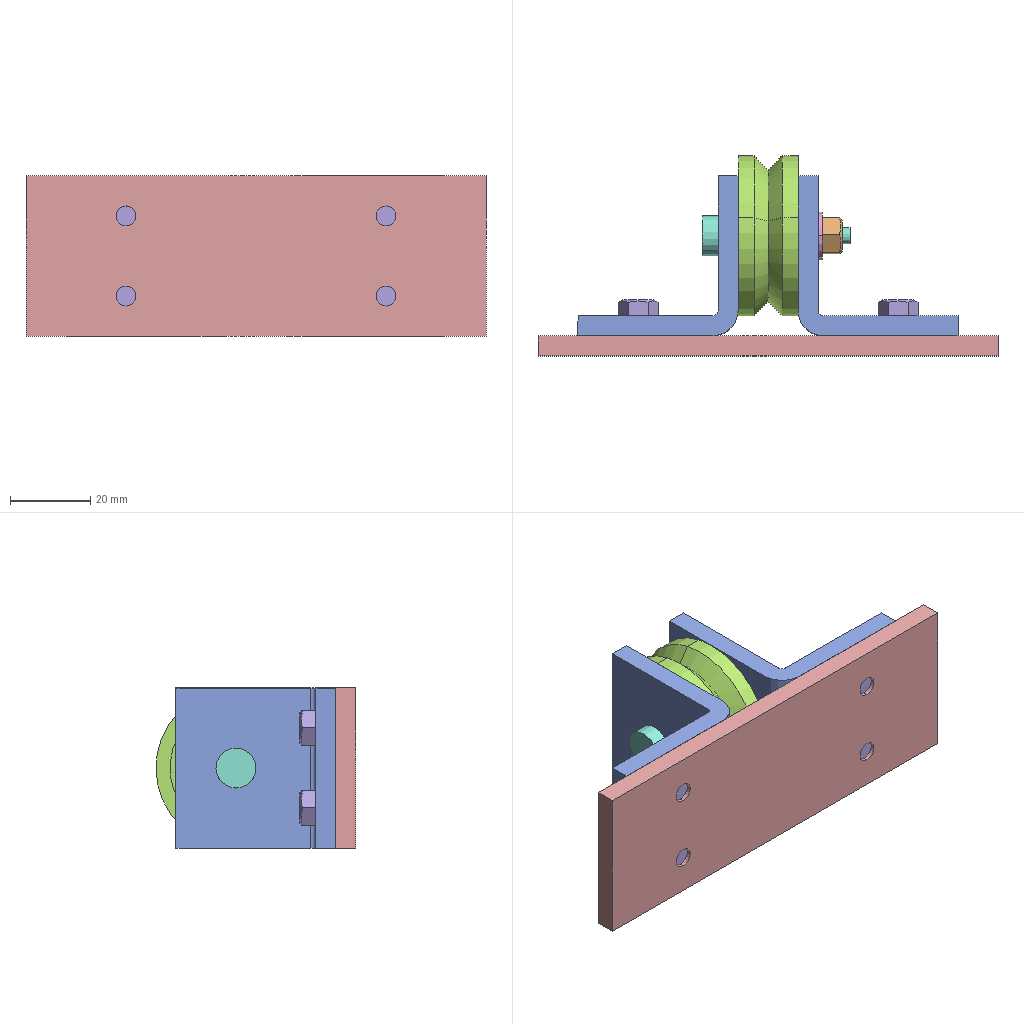Assembly | SolidWorks | 8 different items | 13 placed | box 115 x 50 x 40 mm
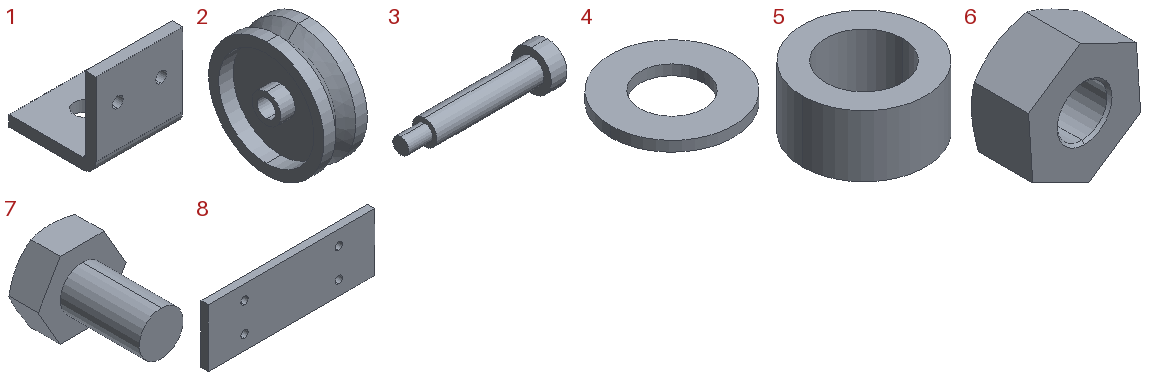Parts list (item | quantity | size | volume | features):
1 | x2 | 40 x 40 x 40 mm | 14089 mm3 | features ICE 2, Extrusion 1
2 | x1 | 15 x 40 x 40 mm | 9172 mm3 | features Revolution 1
3 | x1 | 37 x 10 x 10 mm | 1218 mm3 | features Revolution 1
4 | x1 | 12 x 12 x 1 mm | 82.418 mm3 | features Extrusion 1
5 | x2 | 10 x 10 x 5 mm | 239.301 mm3 | features Extrusion 1
6 | x1 | 8.983 x 5 x 9.976 mm | 257.478 mm3 | features Chamfer 2, Extrusion 1, ICE 1
7 | x4 | 10 x 13 x 8.66 mm | 432.272 mm3 | features ICE 2, Extrusion 1
8 | x1 | 115 x 5 x 40 mm | 22607 mm3 | features Extrusion 1, ICE 1
Mates (type | each side: item.copy, entity, surface, feature):
Coincident | 8.1 face plane Boss-Extrude1 | 1.1 face plane Boss-Extrude1
Concentric | 8.1 face cylinder Cut-Extrude1 | 1.1 face cylinder Cut-Extrude2 | 2 times
Coincident | 8.1 face plane Boss-Extrude1 | 1.2 face plane Boss-Extrude1
Concentric | 8.1 face cylinder Cut-Extrude1 | 1.2 face cylinder Cut-Extrude2 | 2 times
Concentric | 1.2 face cylinder Cut-Extrude1 | 2.1 face cylinder Revolve1
Coincident | 1.2 face plane Boss-Extrude1 | 2.1 face plane Revolve1
Coincident | 1.2 face plane Boss-Extrude1 | 4.1 face plane Boss-Extrude1
Concentric | 1.2 face cylinder Cut-Extrude1 | 4.1 face cylinder Boss-Extrude1
Concentric | 1.1 face cylinder Cut-Extrude1 | 3.1 face cylinder Revolve1
Concentric | 3.1 face cylinder Revolve1 | 6.1 face cylinder Boss-Extrude1
Coincident | 4.1 face plane Boss-Extrude1 | 6.1 face plane Boss-Extrude1
Coincident | 1.1 face plane Boss-Extrude1 | 3.1 face plane Revolve1
Concentric | 1.1 face cylinder Cut-Extrude2 | 7.1 face cylinder Boss-Extrude2
Coincident | 1.1 face plane Boss-Extrude1 | 7.1 face plane Boss-Extrude1
Concentric | 1.1 face cylinder Cut-Extrude2 | 7.2 face cylinder Boss-Extrude2
Coincident | 1.1 face plane Boss-Extrude1 | 7.2 face plane Boss-Extrude1
Coincident | 1.2 face plane Boss-Extrude1 | 7.3 face plane Boss-Extrude1
Concentric | 1.2 face cylinder Cut-Extrude2 | 7.3 face cylinder Boss-Extrude2
Coincident | 1.2 edge | 7.4 face cylinder Boss-Extrude2
Coincident | 1.2 face plane Boss-Extrude1 | 7.4 face plane Boss-Extrude1
Concentric | 3.1 face cylinder Revolve1 | 5.1 face cylinder Boss-Extrude1
Coincident | 3.1 face plane Revolve1 | 5.1 face plane Boss-Extrude1
Concentric | 3.1 face cylinder Revolve1 | 5.2 face cylinder Boss-Extrude1
Coincident | 2.1 face plane Revolve1 | 5.2 face plane Boss-Extrude1